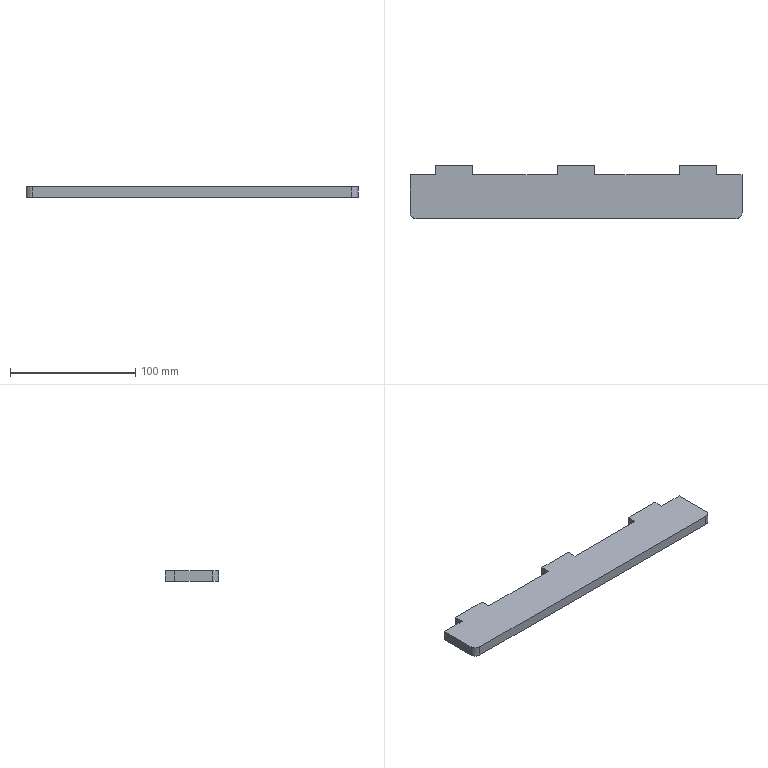Part | SolidWorks | features FlatPattern 1, SMBaseFlange 1, SheetMetal 1 | 1 solid | 20 faces | box 265 x 42.5 x 8 mm | volume 79514 mm3 | plane 18 | cylinder 2 | commonest cylinder face diameters 10 x2
STEP:
#1=CARTESIAN_POINT('',(-87.183,-10.162,0.));
#2=VERTEX_POINT('',#1);
#3=CARTESIAN_POINT('',(-87.183,-40.162,0.));
#4=VERTEX_POINT('',#3);
#5=CARTESIAN_POINT('',(-87.183,-40.162,0.));
#6=DIRECTION('',(0.,-1.,0.));
#7=VECTOR('',#6,1000.);
#8=LINE('',#5,#7);
#9=EDGE_CURVE('',#2,#4,#8,.T.);
#10=ORIENTED_EDGE('',*,*,#9,.F.);
#11=CARTESIAN_POINT('',(-87.183,-10.162,-8.));
#12=VERTEX_POINT('',#11);
#13=CARTESIAN_POINT('',(-87.183,-10.162,-8.));
#14=DIRECTION('',(0.,0.,1.));
#15=VECTOR('',#14,1000.);
#16=LINE('',#13,#15);
#17=EDGE_CURVE('',#12,#2,#16,.T.);
#18=ORIENTED_EDGE('',*,*,#17,.F.);
#19=CARTESIAN_POINT('',(-87.183,-40.162,-8.));
#20=VERTEX_POINT('',#19);
#21=CARTESIAN_POINT('',(-87.183,-40.162,-8.));
#22=DIRECTION('',(0.,-1.,0.));
#23=VECTOR('',#22,1000.);
#24=LINE('',#21,#23);
#25=EDGE_CURVE('',#12,#20,#24,.T.);
#26=ORIENTED_EDGE('',*,*,#25,.T.);
#27=CARTESIAN_POINT('',(-87.183,-40.162,-8.));
#28=DIRECTION('',(0.,0.,1.));
#29=VECTOR('',#28,1000.);
#30=LINE('',#27,#29);
#31=EDGE_CURVE('',#20,#4,#30,.T.);
#32=ORIENTED_EDGE('',*,*,#31,.T.);
#33=EDGE_LOOP('',(#10,#18,#26,#32));
#34=FACE_OUTER_BOUND('',#33,.T.);
#35=CARTESIAN_POINT('',(-87.183,-40.162,-8.));
#36=DIRECTION('',(-1.,0.,0.));
#37=DIRECTION('',(0.,0.,1.));
#38=AXIS2_PLACEMENT_3D('',#35,#36,#37);
#39=PLANE('',#38);
#40=ADVANCED_FACE('',(#34),#39,.T.);
#41=CARTESIAN_POINT('',(-67.183,-10.162,0.));
#42=VERTEX_POINT('',#41);
#43=CARTESIAN_POINT('',(-87.183,-10.162,0.));
#44=DIRECTION('',(-1.,0.,0.));
#45=VECTOR('',#44,1000.);
#46=LINE('',#43,#45);
#47=EDGE_CURVE('',#42,#2,#46,.T.);
#48=ORIENTED_EDGE('',*,*,#47,.F.);
#49=CARTESIAN_POINT('',(-67.183,-10.162,-8.));
#50=VERTEX_POINT('',#49);
#51=CARTESIAN_POINT('',(-67.183,-10.162,-8.));
#52=DIRECTION('',(0.,0.,1.));
#53=VECTOR('',#52,1000.);
#54=LINE('',#51,#53);
#55=EDGE_CURVE('',#50,#42,#54,.T.);
#56=ORIENTED_EDGE('',*,*,#55,.F.);
#57=CARTESIAN_POINT('',(-87.183,-10.162,-8.));
#58=DIRECTION('',(-1.,0.,0.));
#59=VECTOR('',#58,1000.);
#60=LINE('',#57,#59);
#61=EDGE_CURVE('',#50,#12,#60,.T.);
#62=ORIENTED_EDGE('',*,*,#61,.T.);
#63=ORIENTED_EDGE('',*,*,#17,.T.);
#64=EDGE_LOOP('',(#48,#56,#62,#63));
#65=FACE_OUTER_BOUND('',#64,.T.);
#66=CARTESIAN_POINT('',(-87.183,-10.162,-8.));
#67=DIRECTION('',(0.,1.,0.));
#68=DIRECTION('',(-1.,0.,0.));
#69=AXIS2_PLACEMENT_3D('',#66,#67,#68);
#70=PLANE('',#69);
#71=ADVANCED_FACE('',(#65),#70,.T.);
#72=CARTESIAN_POINT('',(-67.183,-2.662,0.));
#73=VERTEX_POINT('',#72);
#74=CARTESIAN_POINT('',(-67.183,-10.162,0.));
#75=DIRECTION('',(0.,-1.,0.));
#76=VECTOR('',#75,1000.);
#77=LINE('',#74,#76);
#78=EDGE_CURVE('',#73,#42,#77,.T.);
#79=ORIENTED_EDGE('',*,*,#78,.F.);
#80=CARTESIAN_POINT('',(-67.183,-2.662,-8.));
#81=VERTEX_POINT('',#80);
#82=CARTESIAN_POINT('',(-67.183,-2.662,-8.));
#83=DIRECTION('',(0.,0.,1.));
#84=VECTOR('',#83,1000.);
#85=LINE('',#82,#84);
#86=EDGE_CURVE('',#81,#73,#85,.T.);
#87=ORIENTED_EDGE('',*,*,#86,.F.);
#88=CARTESIAN_POINT('',(-67.183,-10.162,-8.));
#89=DIRECTION('',(0.,-1.,0.));
#90=VECTOR('',#89,1000.);
#91=LINE('',#88,#90);
#92=EDGE_CURVE('',#81,#50,#91,.T.);
#93=ORIENTED_EDGE('',*,*,#92,.T.);
#94=ORIENTED_EDGE('',*,*,#55,.T.);
#95=EDGE_LOOP('',(#79,#87,#93,#94));
#96=FACE_OUTER_BOUND('',#95,.T.);
#97=CARTESIAN_POINT('',(-67.183,-10.162,-8.));
#98=DIRECTION('',(-1.,0.,0.));
#99=DIRECTION('',(0.,0.,1.));
#100=AXIS2_PLACEMENT_3D('',#97,#98,#99);
#101=PLANE('',#100);
#102=ADVANCED_FACE('',(#96),#101,.T.);
#103=CARTESIAN_POINT('',(-37.183,-2.662,0.));
#104=VERTEX_POINT('',#103);
#105=CARTESIAN_POINT('',(-67.183,-2.662,0.));
#106=DIRECTION('',(-1.,0.,0.));
#107=VECTOR('',#106,1000.);
#108=LINE('',#105,#107);
#109=EDGE_CURVE('',#104,#73,#108,.T.);
#110=ORIENTED_EDGE('',*,*,#109,.F.);
#111=CARTESIAN_POINT('',(-37.183,-2.662,-8.));
#112=VERTEX_POINT('',#111);
#113=CARTESIAN_POINT('',(-37.183,-2.662,-8.));
#114=DIRECTION('',(0.,0.,1.));
#115=VECTOR('',#114,1000.);
#116=LINE('',#113,#115);
#117=EDGE_CURVE('',#112,#104,#116,.T.);
#118=ORIENTED_EDGE('',*,*,#117,.F.);
#119=CARTESIAN_POINT('',(-67.183,-2.662,-8.));
#120=DIRECTION('',(-1.,0.,0.));
#121=VECTOR('',#120,1000.);
#122=LINE('',#119,#121);
#123=EDGE_CURVE('',#112,#81,#122,.T.);
#124=ORIENTED_EDGE('',*,*,#123,.T.);
#125=ORIENTED_EDGE('',*,*,#86,.T.);
#126=EDGE_LOOP('',(#110,#118,#124,#125));
#127=FACE_OUTER_BOUND('',#126,.T.);
#128=CARTESIAN_POINT('',(-67.183,-2.662,-8.));
#129=DIRECTION('',(0.,1.,0.));
#130=DIRECTION('',(0.,0.,1.));
#131=AXIS2_PLACEMENT_3D('',#128,#129,#130);
#132=PLANE('',#131);
#133=ADVANCED_FACE('',(#127),#132,.T.);
#134=CARTESIAN_POINT('',(-37.183,-10.162,0.));
#135=VERTEX_POINT('',#134);
#136=CARTESIAN_POINT('',(-37.183,-2.662,0.));
#137=DIRECTION('',(0.,1.,0.));
#138=VECTOR('',#137,1000.);
#139=LINE('',#136,#138);
#140=EDGE_CURVE('',#135,#104,#139,.T.);
#141=ORIENTED_EDGE('',*,*,#140,.F.);
#142=CARTESIAN_POINT('',(-37.183,-10.162,-8.));
#143=VERTEX_POINT('',#142);
#144=CARTESIAN_POINT('',(-37.183,-10.162,-8.));
#145=DIRECTION('',(0.,0.,1.));
#146=VECTOR('',#145,1000.);
#147=LINE('',#144,#146);
#148=EDGE_CURVE('',#143,#135,#147,.T.);
#149=ORIENTED_EDGE('',*,*,#148,.F.);
#150=CARTESIAN_POINT('',(-37.183,-2.662,-8.));
#151=DIRECTION('',(0.,1.,0.));
#152=VECTOR('',#151,1000.);
#153=LINE('',#150,#152);
#154=EDGE_CURVE('',#143,#112,#153,.T.);
#155=ORIENTED_EDGE('',*,*,#154,.T.);
#156=ORIENTED_EDGE('',*,*,#117,.T.);
#157=EDGE_LOOP('',(#141,#149,#155,#156));
#158=FACE_OUTER_BOUND('',#157,.T.);
#159=CARTESIAN_POINT('',(-37.183,-2.662,-8.));
#160=DIRECTION('',(1.,0.,0.));
#161=DIRECTION('',(0.,0.,-1.));
#162=AXIS2_PLACEMENT_3D('',#159,#160,#161);
#163=PLANE('',#162);
#164=ADVANCED_FACE('',(#158),#163,.T.);
#165=CARTESIAN_POINT('',(30.317,-10.162,0.));
#166=VERTEX_POINT('',#165);
#167=CARTESIAN_POINT('',(-37.183,-10.162,0.));
#168=DIRECTION('',(-1.,0.,0.));
#169=VECTOR('',#168,1000.);
#170=LINE('',#167,#169);
#171=EDGE_CURVE('',#166,#135,#170,.T.);
#172=ORIENTED_EDGE('',*,*,#171,.F.);
#173=CARTESIAN_POINT('',(30.317,-10.162,-8.));
#174=VERTEX_POINT('',#173);
#175=CARTESIAN_POINT('',(30.317,-10.162,-8.));
#176=DIRECTION('',(0.,0.,1.));
#177=VECTOR('',#176,1000.);
#178=LINE('',#175,#177);
#179=EDGE_CURVE('',#174,#166,#178,.T.);
#180=ORIENTED_EDGE('',*,*,#179,.F.);
#181=CARTESIAN_POINT('',(-37.183,-10.162,-8.));
#182=DIRECTION('',(-1.,0.,0.));
#183=VECTOR('',#182,1000.);
#184=LINE('',#181,#183);
#185=EDGE_CURVE('',#174,#143,#184,.T.);
#186=ORIENTED_EDGE('',*,*,#185,.T.);
#187=ORIENTED_EDGE('',*,*,#148,.T.);
#188=EDGE_LOOP('',(#172,#180,#186,#187));
#189=FACE_OUTER_BOUND('',#188,.T.);
#190=CARTESIAN_POINT('',(-37.183,-10.162,-8.));
#191=DIRECTION('',(0.,1.,0.));
#192=DIRECTION('',(-1.,0.,0.));
#193=AXIS2_PLACEMENT_3D('',#190,#191,#192);
#194=PLANE('',#193);
#195=ADVANCED_FACE('',(#189),#194,.T.);
#196=CARTESIAN_POINT('',(30.317,-2.662,0.));
#197=VERTEX_POINT('',#196);
#198=CARTESIAN_POINT('',(30.317,-10.162,0.));
#199=DIRECTION('',(0.,-1.,0.));
#200=VECTOR('',#199,1000.);
#201=LINE('',#198,#200);
#202=EDGE_CURVE('',#197,#166,#201,.T.);
#203=ORIENTED_EDGE('',*,*,#202,.F.);
#204=CARTESIAN_POINT('',(30.317,-2.662,-8.));
#205=VERTEX_POINT('',#204);
#206=CARTESIAN_POINT('',(30.317,-2.662,-8.));
#207=DIRECTION('',(0.,0.,1.));
#208=VECTOR('',#207,1000.);
#209=LINE('',#206,#208);
#210=EDGE_CURVE('',#205,#197,#209,.T.);
#211=ORIENTED_EDGE('',*,*,#210,.F.);
#212=CARTESIAN_POINT('',(30.317,-10.162,-8.));
#213=DIRECTION('',(0.,-1.,0.));
#214=VECTOR('',#213,1000.);
#215=LINE('',#212,#214);
#216=EDGE_CURVE('',#205,#174,#215,.T.);
#217=ORIENTED_EDGE('',*,*,#216,.T.);
#218=ORIENTED_EDGE('',*,*,#179,.T.);
#219=EDGE_LOOP('',(#203,#211,#217,#218));
#220=FACE_OUTER_BOUND('',#219,.T.);
#221=CARTESIAN_POINT('',(30.317,-10.162,-8.));
#222=DIRECTION('',(-1.,0.,0.));
#223=DIRECTION('',(0.,0.,1.));
#224=AXIS2_PLACEMENT_3D('',#221,#222,#223);
#225=PLANE('',#224);
#226=ADVANCED_FACE('',(#220),#225,.T.);
#227=CARTESIAN_POINT('',(60.317,-2.662,0.));
#228=VERTEX_POINT('',#227);
#229=CARTESIAN_POINT('',(30.317,-2.662,0.));
#230=DIRECTION('',(-1.,0.,0.));
#231=VECTOR('',#230,1000.);
#232=LINE('',#229,#231);
#233=EDGE_CURVE('',#228,#197,#232,.T.);
#234=ORIENTED_EDGE('',*,*,#233,.F.);
#235=CARTESIAN_POINT('',(60.317,-2.662,-8.));
#236=VERTEX_POINT('',#235);
#237=CARTESIAN_POINT('',(60.317,-2.662,-8.));
#238=DIRECTION('',(0.,0.,1.));
#239=VECTOR('',#238,1000.);
#240=LINE('',#237,#239);
#241=EDGE_CURVE('',#236,#228,#240,.T.);
#242=ORIENTED_EDGE('',*,*,#241,.F.);
#243=CARTESIAN_POINT('',(30.317,-2.662,-8.));
#244=DIRECTION('',(-1.,0.,0.));
#245=VECTOR('',#244,1000.);
#246=LINE('',#243,#245);
#247=EDGE_CURVE('',#236,#205,#246,.T.);
#248=ORIENTED_EDGE('',*,*,#247,.T.);
#249=ORIENTED_EDGE('',*,*,#210,.T.);
#250=EDGE_LOOP('',(#234,#242,#248,#249));
#251=FACE_OUTER_BOUND('',#250,.T.);
#252=CARTESIAN_POINT('',(30.317,-2.662,-8.));
#253=DIRECTION('',(0.,1.,0.));
#254=DIRECTION('',(0.,0.,1.));
#255=AXIS2_PLACEMENT_3D('',#252,#253,#254);
#256=PLANE('',#255);
#257=ADVANCED_FACE('',(#251),#256,.T.);
#258=CARTESIAN_POINT('',(60.317,-10.162,0.));
#259=VERTEX_POINT('',#258);
#260=CARTESIAN_POINT('',(60.317,-2.662,0.));
#261=DIRECTION('',(0.,1.,0.));
#262=VECTOR('',#261,1000.);
#263=LINE('',#260,#262);
#264=EDGE_CURVE('',#259,#228,#263,.T.);
#265=ORIENTED_EDGE('',*,*,#264,.F.);
#266=CARTESIAN_POINT('',(60.317,-10.162,-8.));
#267=VERTEX_POINT('',#266);
#268=CARTESIAN_POINT('',(60.317,-10.162,-8.));
#269=DIRECTION('',(0.,0.,1.));
#270=VECTOR('',#269,1000.);
#271=LINE('',#268,#270);
#272=EDGE_CURVE('',#267,#259,#271,.T.);
#273=ORIENTED_EDGE('',*,*,#272,.F.);
#274=CARTESIAN_POINT('',(60.317,-2.662,-8.));
#275=DIRECTION('',(0.,1.,0.));
#276=VECTOR('',#275,1000.);
#277=LINE('',#274,#276);
#278=EDGE_CURVE('',#267,#236,#277,.T.);
#279=ORIENTED_EDGE('',*,*,#278,.T.);
#280=ORIENTED_EDGE('',*,*,#241,.T.);
#281=EDGE_LOOP('',(#265,#273,#279,#280));
#282=FACE_OUTER_BOUND('',#281,.T.);
#283=CARTESIAN_POINT('',(60.317,-2.662,-8.));
#284=DIRECTION('',(1.,0.,0.));
#285=DIRECTION('',(0.,0.,-1.));
#286=AXIS2_PLACEMENT_3D('',#283,#284,#285);
#287=PLANE('',#286);
#288=ADVANCED_FACE('',(#282),#287,.T.);
#289=CARTESIAN_POINT('',(127.817,-10.162,0.));
#290=VERTEX_POINT('',#289);
#291=CARTESIAN_POINT('',(60.317,-10.162,0.));
#292=DIRECTION('',(-1.,0.,0.));
#293=VECTOR('',#292,1000.);
#294=LINE('',#291,#293);
#295=EDGE_CURVE('',#290,#259,#294,.T.);
#296=ORIENTED_EDGE('',*,*,#295,.F.);
#297=CARTESIAN_POINT('',(127.817,-10.162,-8.));
#298=VERTEX_POINT('',#297);
#299=CARTESIAN_POINT('',(127.817,-10.162,-8.));
#300=DIRECTION('',(0.,0.,1.));
#301=VECTOR('',#300,1000.);
#302=LINE('',#299,#301);
#303=EDGE_CURVE('',#298,#290,#302,.T.);
#304=ORIENTED_EDGE('',*,*,#303,.F.);
#305=CARTESIAN_POINT('',(60.317,-10.162,-8.));
#306=DIRECTION('',(-1.,0.,0.));
#307=VECTOR('',#306,1000.);
#308=LINE('',#305,#307);
#309=EDGE_CURVE('',#298,#267,#308,.T.);
#310=ORIENTED_EDGE('',*,*,#309,.T.);
#311=ORIENTED_EDGE('',*,*,#272,.T.);
#312=EDGE_LOOP('',(#296,#304,#310,#311));
#313=FACE_OUTER_BOUND('',#312,.T.);
#314=CARTESIAN_POINT('',(60.317,-10.162,-8.));
#315=DIRECTION('',(0.,1.,0.));
#316=DIRECTION('',(-1.,0.,0.));
#317=AXIS2_PLACEMENT_3D('',#314,#315,#316);
#318=PLANE('',#317);
#319=ADVANCED_FACE('',(#313),#318,.T.);
#320=CARTESIAN_POINT('',(127.817,-2.662,0.));
#321=VERTEX_POINT('',#320);
#322=CARTESIAN_POINT('',(127.817,-10.162,0.));
#323=DIRECTION('',(0.,-1.,0.));
#324=VECTOR('',#323,1000.);
#325=LINE('',#322,#324);
#326=EDGE_CURVE('',#321,#290,#325,.T.);
#327=ORIENTED_EDGE('',*,*,#326,.F.);
#328=CARTESIAN_POINT('',(127.817,-2.662,-8.));
#329=VERTEX_POINT('',#328);
#330=CARTESIAN_POINT('',(127.817,-2.662,-8.));
#331=DIRECTION('',(0.,0.,1.));
#332=VECTOR('',#331,1000.);
#333=LINE('',#330,#332);
#334=EDGE_CURVE('',#329,#321,#333,.T.);
#335=ORIENTED_EDGE('',*,*,#334,.F.);
#336=CARTESIAN_POINT('',(127.817,-10.162,-8.));
#337=DIRECTION('',(0.,-1.,0.));
#338=VECTOR('',#337,1000.);
#339=LINE('',#336,#338);
#340=EDGE_CURVE('',#329,#298,#339,.T.);
#341=ORIENTED_EDGE('',*,*,#340,.T.);
#342=ORIENTED_EDGE('',*,*,#303,.T.);
#343=EDGE_LOOP('',(#327,#335,#341,#342));
#344=FACE_OUTER_BOUND('',#343,.T.);
#345=CARTESIAN_POINT('',(127.817,-10.162,-8.));
#346=DIRECTION('',(-1.,0.,0.));
#347=DIRECTION('',(0.,0.,1.));
#348=AXIS2_PLACEMENT_3D('',#345,#346,#347);
#349=PLANE('',#348);
#350=ADVANCED_FACE('',(#344),#349,.T.);
#351=CARTESIAN_POINT('',(157.817,-2.662,0.));
#352=VERTEX_POINT('',#351);
#353=CARTESIAN_POINT('',(127.817,-2.662,0.));
#354=DIRECTION('',(-1.,0.,0.));
#355=VECTOR('',#354,1000.);
#356=LINE('',#353,#355);
#357=EDGE_CURVE('',#352,#321,#356,.T.);
#358=ORIENTED_EDGE('',*,*,#357,.F.);
#359=CARTESIAN_POINT('',(157.817,-2.662,-8.));
#360=VERTEX_POINT('',#359);
#361=CARTESIAN_POINT('',(157.817,-2.662,-8.));
#362=DIRECTION('',(0.,0.,1.));
#363=VECTOR('',#362,1000.);
#364=LINE('',#361,#363);
#365=EDGE_CURVE('',#360,#352,#364,.T.);
#366=ORIENTED_EDGE('',*,*,#365,.F.);
#367=CARTESIAN_POINT('',(127.817,-2.662,-8.));
#368=DIRECTION('',(-1.,0.,0.));
#369=VECTOR('',#368,1000.);
#370=LINE('',#367,#369);
#371=EDGE_CURVE('',#360,#329,#370,.T.);
#372=ORIENTED_EDGE('',*,*,#371,.T.);
#373=ORIENTED_EDGE('',*,*,#334,.T.);
#374=EDGE_LOOP('',(#358,#366,#372,#373));
#375=FACE_OUTER_BOUND('',#374,.T.);
#376=CARTESIAN_POINT('',(127.817,-2.662,-8.));
#377=DIRECTION('',(0.,1.,0.));
#378=DIRECTION('',(0.,0.,1.));
#379=AXIS2_PLACEMENT_3D('',#376,#377,#378);
#380=PLANE('',#379);
#381=ADVANCED_FACE('',(#375),#380,.T.);
#382=CARTESIAN_POINT('',(157.817,-10.162,0.));
#383=VERTEX_POINT('',#382);
#384=CARTESIAN_POINT('',(157.817,-2.662,0.));
#385=DIRECTION('',(0.,1.,0.));
#386=VECTOR('',#385,1000.);
#387=LINE('',#384,#386);
#388=EDGE_CURVE('',#383,#352,#387,.T.);
#389=ORIENTED_EDGE('',*,*,#388,.F.);
#390=CARTESIAN_POINT('',(157.817,-10.162,-8.));
#391=VERTEX_POINT('',#390);
#392=CARTESIAN_POINT('',(157.817,-10.162,-8.));
#393=DIRECTION('',(0.,0.,1.));
#394=VECTOR('',#393,1000.);
#395=LINE('',#392,#394);
#396=EDGE_CURVE('',#391,#383,#395,.T.);
#397=ORIENTED_EDGE('',*,*,#396,.F.);
#398=CARTESIAN_POINT('',(157.817,-2.662,-8.));
#399=DIRECTION('',(0.,1.,0.));
#400=VECTOR('',#399,1000.);
#401=LINE('',#398,#400);
#402=EDGE_CURVE('',#391,#360,#401,.T.);
#403=ORIENTED_EDGE('',*,*,#402,.T.);
#404=ORIENTED_EDGE('',*,*,#365,.T.);
#405=EDGE_LOOP('',(#389,#397,#403,#404));
#406=FACE_OUTER_BOUND('',#405,.T.);
#407=CARTESIAN_POINT('',(157.817,-2.662,-8.));
#408=DIRECTION('',(1.,0.,0.));
#409=DIRECTION('',(0.,0.,-1.));
#410=AXIS2_PLACEMENT_3D('',#407,#408,#409);
#411=PLANE('',#410);
#412=ADVANCED_FACE('',(#406),#411,.T.);
#413=CARTESIAN_POINT('',(177.817,-10.162,0.));
#414=VERTEX_POINT('',#413);
#415=CARTESIAN_POINT('',(157.817,-10.162,0.));
#416=DIRECTION('',(-1.,0.,0.));
#417=VECTOR('',#416,1000.);
#418=LINE('',#415,#417);
#419=EDGE_CURVE('',#414,#383,#418,.T.);
#420=ORIENTED_EDGE('',*,*,#419,.F.);
#421=CARTESIAN_POINT('',(177.817,-10.162,-8.));
#422=VERTEX_POINT('',#421);
#423=CARTESIAN_POINT('',(177.817,-10.162,-8.));
#424=DIRECTION('',(0.,0.,1.));
#425=VECTOR('',#424,1000.);
#426=LINE('',#423,#425);
#427=EDGE_CURVE('',#422,#414,#426,.T.);
#428=ORIENTED_EDGE('',*,*,#427,.F.);
#429=CARTESIAN_POINT('',(157.817,-10.162,-8.));
#430=DIRECTION('',(-1.,0.,0.));
#431=VECTOR('',#430,1000.);
#432=LINE('',#429,#431);
#433=EDGE_CURVE('',#422,#391,#432,.T.);
#434=ORIENTED_EDGE('',*,*,#433,.T.);
#435=ORIENTED_EDGE('',*,*,#396,.T.);
#436=EDGE_LOOP('',(#420,#428,#434,#435));
#437=FACE_OUTER_BOUND('',#436,.T.);
#438=CARTESIAN_POINT('',(157.817,-10.162,-8.));
#439=DIRECTION('',(0.,1.,0.));
#440=DIRECTION('',(0.,0.,1.));
#441=AXIS2_PLACEMENT_3D('',#438,#439,#440);
#442=PLANE('',#441);
#443=ADVANCED_FACE('',(#437),#442,.T.);
#444=CARTESIAN_POINT('',(177.817,-40.162,0.));
#445=VERTEX_POINT('',#444);
#446=CARTESIAN_POINT('',(177.817,-10.162,0.));
#447=DIRECTION('',(0.,1.,0.));
#448=VECTOR('',#447,1000.);
#449=LINE('',#446,#448);
#450=EDGE_CURVE('',#445,#414,#449,.T.);
#451=ORIENTED_EDGE('',*,*,#450,.F.);
#452=CARTESIAN_POINT('',(177.817,-40.162,-8.));
#453=VERTEX_POINT('',#452);
#454=CARTESIAN_POINT('',(177.817,-40.162,-8.));
#455=DIRECTION('',(0.,0.,1.));
#456=VECTOR('',#455,1000.);
#457=LINE('',#454,#456);
#458=EDGE_CURVE('',#453,#445,#457,.T.);
#459=ORIENTED_EDGE('',*,*,#458,.F.);
#460=CARTESIAN_POINT('',(177.817,-10.162,-8.));
#461=DIRECTION('',(0.,1.,0.));
#462=VECTOR('',#461,1000.);
#463=LINE('',#460,#462);
#464=EDGE_CURVE('',#453,#422,#463,.T.);
#465=ORIENTED_EDGE('',*,*,#464,.T.);
#466=ORIENTED_EDGE('',*,*,#427,.T.);
#467=EDGE_LOOP('',(#451,#459,#465,#466));
#468=FACE_OUTER_BOUND('',#467,.T.);
#469=CARTESIAN_POINT('',(177.817,-10.162,-8.));
#470=DIRECTION('',(1.,0.,0.));
#471=DIRECTION('',(0.,0.,-1.));
#472=AXIS2_PLACEMENT_3D('',#469,#470,#471);
#473=PLANE('',#472);
#474=ADVANCED_FACE('',(#468),#473,.T.);
#475=CARTESIAN_POINT('',(172.817,-45.162,0.));
#476=VERTEX_POINT('',#475);
#477=CARTESIAN_POINT('',(172.817,-40.162,0.));
#478=DIRECTION('',(0.,0.,1.));
#479=DIRECTION('',(-1.,0.,0.));
#480=AXIS2_PLACEMENT_3D('',#477,#478,#479);
#481=CIRCLE('',#480,5.);
#482=EDGE_CURVE('',#476,#445,#481,.T.);
#483=ORIENTED_EDGE('',*,*,#482,.F.);
#484=CARTESIAN_POINT('',(172.817,-45.162,-8.));
#485=VERTEX_POINT('',#484);
#486=CARTESIAN_POINT('',(172.817,-45.162,-8.));
#487=DIRECTION('',(0.,0.,1.));
#488=VECTOR('',#487,1000.);
#489=LINE('',#486,#488);
#490=EDGE_CURVE('',#485,#476,#489,.T.);
#491=ORIENTED_EDGE('',*,*,#490,.F.);
#492=CARTESIAN_POINT('',(172.817,-40.162,-8.));
#493=DIRECTION('',(0.,0.,1.));
#494=DIRECTION('',(-1.,0.,0.));
#495=AXIS2_PLACEMENT_3D('',#492,#493,#494);
#496=CIRCLE('',#495,5.);
#497=EDGE_CURVE('',#485,#453,#496,.T.);
#498=ORIENTED_EDGE('',*,*,#497,.T.);
#499=ORIENTED_EDGE('',*,*,#458,.T.);
#500=EDGE_LOOP('',(#483,#491,#498,#499));
#501=FACE_OUTER_BOUND('',#500,.T.);
#502=CARTESIAN_POINT('',(172.817,-40.162,-8.));
#503=DIRECTION('',(0.,0.,1.));
#504=DIRECTION('',(1.,0.,0.));
#505=AXIS2_PLACEMENT_3D('',#502,#503,#504);
#506=CYLINDRICAL_SURFACE('',#505,5.);
#507=ADVANCED_FACE('',(#501),#506,.T.);
#508=CARTESIAN_POINT('',(-82.183,-45.162,0.));
#509=VERTEX_POINT('',#508);
#510=CARTESIAN_POINT('',(172.817,-45.162,0.));
#511=DIRECTION('',(1.,0.,0.));
#512=VECTOR('',#511,1000.);
#513=LINE('',#510,#512);
#514=EDGE_CURVE('',#509,#476,#513,.T.);
#515=ORIENTED_EDGE('',*,*,#514,.F.);
#516=CARTESIAN_POINT('',(-82.183,-45.162,-8.));
#517=VERTEX_POINT('',#516);
#518=CARTESIAN_POINT('',(-82.183,-45.162,-8.));
#519=DIRECTION('',(0.,0.,1.));
#520=VECTOR('',#519,1000.);
#521=LINE('',#518,#520);
#522=EDGE_CURVE('',#517,#509,#521,.T.);
#523=ORIENTED_EDGE('',*,*,#522,.F.);
#524=CARTESIAN_POINT('',(172.817,-45.162,-8.));
#525=DIRECTION('',(1.,0.,0.));
#526=VECTOR('',#525,1000.);
#527=LINE('',#524,#526);
#528=EDGE_CURVE('',#517,#485,#527,.T.);
#529=ORIENTED_EDGE('',*,*,#528,.T.);
#530=ORIENTED_EDGE('',*,*,#490,.T.);
#531=EDGE_LOOP('',(#515,#523,#529,#530));
#532=FACE_OUTER_BOUND('',#531,.T.);
#533=CARTESIAN_POINT('',(172.817,-45.162,-8.));
#534=DIRECTION('',(0.,-1.,0.));
#535=DIRECTION('',(1.,0.,0.));
#536=AXIS2_PLACEMENT_3D('',#533,#534,#535);
#537=PLANE('',#536);
#538=ADVANCED_FACE('',(#532),#537,.T.);
#539=CARTESIAN_POINT('',(-82.183,-40.162,0.));
#540=DIRECTION('',(0.,0.,1.));
#541=DIRECTION('',(-1.,0.,0.));
#542=AXIS2_PLACEMENT_3D('',#539,#540,#541);
#543=CIRCLE('',#542,5.);
#544=EDGE_CURVE('',#4,#509,#543,.T.);
#545=ORIENTED_EDGE('',*,*,#544,.F.);
#546=ORIENTED_EDGE('',*,*,#31,.F.);
#547=CARTESIAN_POINT('',(-82.183,-40.162,-8.));
#548=DIRECTION('',(0.,0.,1.));
#549=DIRECTION('',(-1.,0.,0.));
#550=AXIS2_PLACEMENT_3D('',#547,#548,#549);
#551=CIRCLE('',#550,5.);
#552=EDGE_CURVE('',#20,#517,#551,.T.);
#553=ORIENTED_EDGE('',*,*,#552,.T.);
#554=ORIENTED_EDGE('',*,*,#522,.T.);
#555=EDGE_LOOP('',(#545,#546,#553,#554));
#556=FACE_OUTER_BOUND('',#555,.T.);
#557=CARTESIAN_POINT('',(-82.183,-40.162,-8.));
#558=DIRECTION('',(0.,0.,1.));
#559=DIRECTION('',(1.,0.,0.));
#560=AXIS2_PLACEMENT_3D('',#557,#558,#559);
#561=CYLINDRICAL_SURFACE('',#560,5.);
#562=ADVANCED_FACE('',(#556),#561,.T.);
#563=ORIENTED_EDGE('',*,*,#25,.F.);
#564=ORIENTED_EDGE('',*,*,#61,.F.);
#565=ORIENTED_EDGE('',*,*,#92,.F.);
#566=ORIENTED_EDGE('',*,*,#123,.F.);
#567=ORIENTED_EDGE('',*,*,#154,.F.);
#568=ORIENTED_EDGE('',*,*,#185,.F.);
#569=ORIENTED_EDGE('',*,*,#216,.F.);
#570=ORIENTED_EDGE('',*,*,#247,.F.);
#571=ORIENTED_EDGE('',*,*,#278,.F.);
#572=ORIENTED_EDGE('',*,*,#309,.F.);
#573=ORIENTED_EDGE('',*,*,#340,.F.);
#574=ORIENTED_EDGE('',*,*,#371,.F.);
#575=ORIENTED_EDGE('',*,*,#402,.F.);
#576=ORIENTED_EDGE('',*,*,#433,.F.);
#577=ORIENTED_EDGE('',*,*,#464,.F.);
#578=ORIENTED_EDGE('',*,*,#497,.F.);
#579=ORIENTED_EDGE('',*,*,#528,.F.);
#580=ORIENTED_EDGE('',*,*,#552,.F.);
#581=EDGE_LOOP('',(#563,#564,#565,#566,#567,#568,#569,#570,#571,#572,#573,#574,#575,#576,#577,#578,#579,#580));
#582=FACE_OUTER_BOUND('',#581,.T.);
#583=CARTESIAN_POINT('',(172.817,-40.162,-8.));
#584=DIRECTION('',(0.,0.,-1.));
#585=DIRECTION('',(-1.,0.,0.));
#586=AXIS2_PLACEMENT_3D('',#583,#584,#585);
#587=PLANE('',#586);
#588=ADVANCED_FACE('',(#582),#587,.T.);
#589=ORIENTED_EDGE('',*,*,#9,.T.);
#590=ORIENTED_EDGE('',*,*,#544,.T.);
#591=ORIENTED_EDGE('',*,*,#514,.T.);
#592=ORIENTED_EDGE('',*,*,#482,.T.);
#593=ORIENTED_EDGE('',*,*,#450,.T.);
#594=ORIENTED_EDGE('',*,*,#419,.T.);
#595=ORIENTED_EDGE('',*,*,#388,.T.);
#596=ORIENTED_EDGE('',*,*,#357,.T.);
#597=ORIENTED_EDGE('',*,*,#326,.T.);
#598=ORIENTED_EDGE('',*,*,#295,.T.);
#599=ORIENTED_EDGE('',*,*,#264,.T.);
#600=ORIENTED_EDGE('',*,*,#233,.T.);
#601=ORIENTED_EDGE('',*,*,#202,.T.);
#602=ORIENTED_EDGE('',*,*,#171,.T.);
#603=ORIENTED_EDGE('',*,*,#140,.T.);
#604=ORIENTED_EDGE('',*,*,#109,.T.);
#605=ORIENTED_EDGE('',*,*,#78,.T.);
#606=ORIENTED_EDGE('',*,*,#47,.T.);
#607=EDGE_LOOP('',(#589,#590,#591,#592,#593,#594,#595,#596,#597,#598,#599,#600,#601,#602,#603,#604,#605,#606));
#608=FACE_OUTER_BOUND('',#607,.T.);
#609=CARTESIAN_POINT('',(172.817,-40.162,0.));
#610=DIRECTION('',(0.,0.,-1.));
#611=DIRECTION('',(-1.,0.,0.));
#612=AXIS2_PLACEMENT_3D('',#609,#610,#611);
#613=PLANE('',#612);
#614=ADVANCED_FACE('',(#608),#613,.F.);
#615=CLOSED_SHELL('',(#40,#71,#102,#133,#164,#195,#226,#257,#288,#319,#350,#381,#412,#443,#474,#507,#538,#562,#588,#614));
#616=MANIFOLD_SOLID_BREP('',#615);
#617=CARTESIAN_POINT('',(0.,0.,0.));
#618=DIRECTION('',(0.,0.,1.));
#619=DIRECTION('',(1.,0.,0.));
#620=AXIS2_PLACEMENT_3D('',#617,#618,#619);
#621=(LENGTH_UNIT()NAMED_UNIT(*)SI_UNIT(.MILLI.,.METRE.));
#622=UNCERTAINTY_MEASURE_WITH_UNIT(LENGTH_MEASURE(0.00001),#621,'','');
#623=(NAMED_UNIT(*)PLANE_ANGLE_UNIT()SI_UNIT($,.RADIAN.));
#624=(NAMED_UNIT(*)SI_UNIT($,.STERADIAN.)SOLID_ANGLE_UNIT());
#625=(GEOMETRIC_REPRESENTATION_CONTEXT(3)GLOBAL_UNCERTAINTY_ASSIGNED_CONTEXT((#622))GLOBAL_UNIT_ASSIGNED_CONTEXT((#621,#623,#624))REPRESENTATION_CONTEXT('',''));
#626=ADVANCED_BREP_SHAPE_REPRESENTATION('',(#616,#620),#625);